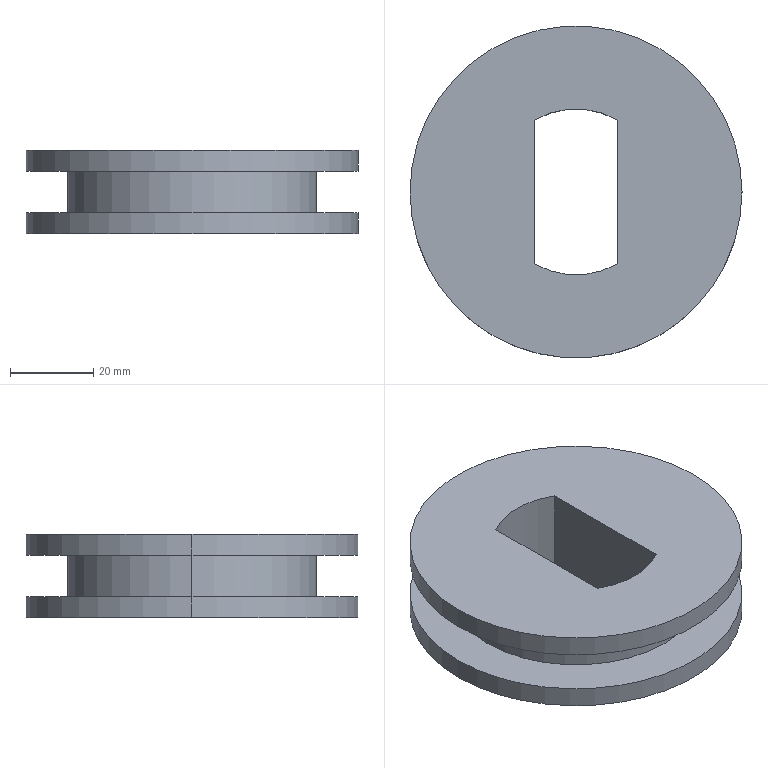Part | SolidWorks | 1 solid | 14 faces | box 80 x 80 x 20 mm | volume 63234 mm3 | cylinder 8 | plane 6 | commonest cylinder face diameters 80 x4 40 x2 60 x2
STEP:
#1=CARTESIAN_POINT('',(30.,0.,-5.));
#2=VERTEX_POINT('',#1);
#3=CARTESIAN_POINT('',(-30.,0.,-5.));
#4=VERTEX_POINT('',#3);
#5=CARTESIAN_POINT('',(0.,0.,-5.));
#6=DIRECTION('',(0.,0.,1.));
#7=DIRECTION('',(1.,0.,0.));
#8=AXIS2_PLACEMENT_3D('',#5,#6,#7);
#9=CIRCLE('',#8,30.);
#10=EDGE_CURVE('',#2,#4,#9,.T.);
#11=ORIENTED_EDGE('',*,*,#10,.T.);
#12=CARTESIAN_POINT('',(-30.,0.,5.));
#13=VERTEX_POINT('',#12);
#14=CARTESIAN_POINT('',(-30.,0.,10.));
#15=DIRECTION('',(0.,0.,1.));
#16=VECTOR('',#15,1000.);
#17=LINE('',#14,#16);
#18=EDGE_CURVE('',#4,#13,#17,.T.);
#19=ORIENTED_EDGE('',*,*,#18,.T.);
#20=CARTESIAN_POINT('',(30.,0.,5.));
#21=VERTEX_POINT('',#20);
#22=CARTESIAN_POINT('',(0.,0.,5.));
#23=DIRECTION('',(0.,0.,1.));
#24=DIRECTION('',(1.,0.,0.));
#25=AXIS2_PLACEMENT_3D('',#22,#23,#24);
#26=CIRCLE('',#25,30.);
#27=EDGE_CURVE('',#21,#13,#26,.T.);
#28=ORIENTED_EDGE('',*,*,#27,.F.);
#29=CARTESIAN_POINT('',(30.,0.,10.));
#30=DIRECTION('',(0.,0.,1.));
#31=VECTOR('',#30,1000.);
#32=LINE('',#29,#31);
#33=EDGE_CURVE('',#2,#21,#32,.T.);
#34=ORIENTED_EDGE('',*,*,#33,.F.);
#35=EDGE_LOOP('',(#11,#19,#28,#34));
#36=FACE_OUTER_BOUND('',#35,.T.);
#37=CARTESIAN_POINT('',(0.,0.,10.));
#38=DIRECTION('',(0.,0.,1.));
#39=DIRECTION('',(1.,0.,0.));
#40=AXIS2_PLACEMENT_3D('',#37,#38,#39);
#41=CYLINDRICAL_SURFACE('',#40,30.);
#42=ADVANCED_FACE('',(#36),#41,.T.);
#43=CARTESIAN_POINT('',(40.,0.,10.));
#44=VERTEX_POINT('',#43);
#45=CARTESIAN_POINT('',(-40.,0.,10.));
#46=VERTEX_POINT('',#45);
#47=CARTESIAN_POINT('',(0.,0.,10.));
#48=DIRECTION('',(0.,0.,1.));
#49=DIRECTION('',(1.,0.,0.));
#50=AXIS2_PLACEMENT_3D('',#47,#48,#49);
#51=CIRCLE('',#50,40.);
#52=EDGE_CURVE('',#44,#46,#51,.T.);
#53=ORIENTED_EDGE('',*,*,#52,.F.);
#54=CARTESIAN_POINT('',(40.,0.,5.));
#55=VERTEX_POINT('',#54);
#56=CARTESIAN_POINT('',(40.,0.,10.));
#57=DIRECTION('',(0.,0.,-1.));
#58=VECTOR('',#57,1000.);
#59=LINE('',#56,#58);
#60=EDGE_CURVE('',#44,#55,#59,.T.);
#61=ORIENTED_EDGE('',*,*,#60,.T.);
#62=CARTESIAN_POINT('',(-40.,0.,5.));
#63=VERTEX_POINT('',#62);
#64=CARTESIAN_POINT('',(0.,0.,5.));
#65=DIRECTION('',(0.,0.,-1.));
#66=DIRECTION('',(-1.,0.,0.));
#67=AXIS2_PLACEMENT_3D('',#64,#65,#66);
#68=CIRCLE('',#67,40.);
#69=EDGE_CURVE('',#63,#55,#68,.T.);
#70=ORIENTED_EDGE('',*,*,#69,.F.);
#71=CARTESIAN_POINT('',(-40.,0.,10.));
#72=DIRECTION('',(0.,0.,-1.));
#73=VECTOR('',#72,1000.);
#74=LINE('',#71,#73);
#75=EDGE_CURVE('',#46,#63,#74,.T.);
#76=ORIENTED_EDGE('',*,*,#75,.F.);
#77=EDGE_LOOP('',(#53,#61,#70,#76));
#78=FACE_OUTER_BOUND('',#77,.T.);
#79=CARTESIAN_POINT('',(0.,0.,10.));
#80=DIRECTION('',(0.,0.,-1.));
#81=DIRECTION('',(-1.,0.,0.));
#82=AXIS2_PLACEMENT_3D('',#79,#80,#81);
#83=CYLINDRICAL_SURFACE('',#82,40.);
#84=ADVANCED_FACE('',(#78),#83,.T.);
#85=CARTESIAN_POINT('',(40.,0.,-5.));
#86=VERTEX_POINT('',#85);
#87=CARTESIAN_POINT('',(-40.,0.,-5.));
#88=VERTEX_POINT('',#87);
#89=CARTESIAN_POINT('',(0.,0.,-5.));
#90=DIRECTION('',(0.,0.,1.));
#91=DIRECTION('',(1.,0.,0.));
#92=AXIS2_PLACEMENT_3D('',#89,#90,#91);
#93=CIRCLE('',#92,40.);
#94=EDGE_CURVE('',#86,#88,#93,.T.);
#95=ORIENTED_EDGE('',*,*,#94,.F.);
#96=CARTESIAN_POINT('',(40.,0.,-10.));
#97=VERTEX_POINT('',#96);
#98=CARTESIAN_POINT('',(40.,0.,10.));
#99=DIRECTION('',(0.,0.,-1.));
#100=VECTOR('',#99,1000.);
#101=LINE('',#98,#100);
#102=EDGE_CURVE('',#86,#97,#101,.T.);
#103=ORIENTED_EDGE('',*,*,#102,.T.);
#104=CARTESIAN_POINT('',(-40.,0.,-10.));
#105=VERTEX_POINT('',#104);
#106=CARTESIAN_POINT('',(0.,0.,-10.));
#107=DIRECTION('',(0.,0.,1.));
#108=DIRECTION('',(1.,0.,0.));
#109=AXIS2_PLACEMENT_3D('',#106,#107,#108);
#110=CIRCLE('',#109,40.);
#111=EDGE_CURVE('',#97,#105,#110,.T.);
#112=ORIENTED_EDGE('',*,*,#111,.T.);
#113=CARTESIAN_POINT('',(-40.,0.,10.));
#114=DIRECTION('',(0.,0.,-1.));
#115=VECTOR('',#114,1000.);
#116=LINE('',#113,#115);
#117=EDGE_CURVE('',#88,#105,#116,.T.);
#118=ORIENTED_EDGE('',*,*,#117,.F.);
#119=EDGE_LOOP('',(#95,#103,#112,#118));
#120=FACE_OUTER_BOUND('',#119,.T.);
#121=CARTESIAN_POINT('',(0.,0.,10.));
#122=DIRECTION('',(0.,0.,-1.));
#123=DIRECTION('',(-1.,0.,0.));
#124=AXIS2_PLACEMENT_3D('',#121,#122,#123);
#125=CYLINDRICAL_SURFACE('',#124,40.);
#126=ADVANCED_FACE('',(#120),#125,.T.);
#127=ORIENTED_EDGE('',*,*,#102,.F.);
#128=CARTESIAN_POINT('',(0.,0.,-5.));
#129=DIRECTION('',(0.,0.,1.));
#130=DIRECTION('',(1.,0.,0.));
#131=AXIS2_PLACEMENT_3D('',#128,#129,#130);
#132=CIRCLE('',#131,40.);
#133=EDGE_CURVE('',#88,#86,#132,.T.);
#134=ORIENTED_EDGE('',*,*,#133,.F.);
#135=ORIENTED_EDGE('',*,*,#117,.T.);
#136=CARTESIAN_POINT('',(0.,0.,-10.));
#137=DIRECTION('',(0.,0.,1.));
#138=DIRECTION('',(1.,0.,0.));
#139=AXIS2_PLACEMENT_3D('',#136,#137,#138);
#140=CIRCLE('',#139,40.);
#141=EDGE_CURVE('',#105,#97,#140,.T.);
#142=ORIENTED_EDGE('',*,*,#141,.T.);
#143=EDGE_LOOP('',(#127,#134,#135,#142));
#144=FACE_OUTER_BOUND('',#143,.T.);
#145=CARTESIAN_POINT('',(0.,0.,10.));
#146=DIRECTION('',(0.,0.,-1.));
#147=DIRECTION('',(-1.,0.,0.));
#148=AXIS2_PLACEMENT_3D('',#145,#146,#147);
#149=CYLINDRICAL_SURFACE('',#148,40.);
#150=ADVANCED_FACE('',(#144),#149,.T.);
#151=ORIENTED_EDGE('',*,*,#60,.F.);
#152=CARTESIAN_POINT('',(0.,0.,10.));
#153=DIRECTION('',(0.,0.,1.));
#154=DIRECTION('',(1.,0.,0.));
#155=AXIS2_PLACEMENT_3D('',#152,#153,#154);
#156=CIRCLE('',#155,40.);
#157=EDGE_CURVE('',#46,#44,#156,.T.);
#158=ORIENTED_EDGE('',*,*,#157,.F.);
#159=ORIENTED_EDGE('',*,*,#75,.T.);
#160=CARTESIAN_POINT('',(0.,0.,5.));
#161=DIRECTION('',(0.,0.,-1.));
#162=DIRECTION('',(-1.,0.,0.));
#163=AXIS2_PLACEMENT_3D('',#160,#161,#162);
#164=CIRCLE('',#163,40.);
#165=EDGE_CURVE('',#55,#63,#164,.T.);
#166=ORIENTED_EDGE('',*,*,#165,.F.);
#167=EDGE_LOOP('',(#151,#158,#159,#166));
#168=FACE_OUTER_BOUND('',#167,.T.);
#169=CARTESIAN_POINT('',(0.,0.,10.));
#170=DIRECTION('',(0.,0.,-1.));
#171=DIRECTION('',(-1.,0.,0.));
#172=AXIS2_PLACEMENT_3D('',#169,#170,#171);
#173=CYLINDRICAL_SURFACE('',#172,40.);
#174=ADVANCED_FACE('',(#168),#173,.T.);
#175=CARTESIAN_POINT('',(10.,17.321,-10.));
#176=VERTEX_POINT('',#175);
#177=CARTESIAN_POINT('',(-10.,17.321,-10.));
#178=VERTEX_POINT('',#177);
#179=CARTESIAN_POINT('',(0.,0.,-10.));
#180=DIRECTION('',(0.,0.,1.));
#181=DIRECTION('',(1.,0.,0.));
#182=AXIS2_PLACEMENT_3D('',#179,#180,#181);
#183=CIRCLE('',#182,20.);
#184=EDGE_CURVE('',#176,#178,#183,.T.);
#185=ORIENTED_EDGE('',*,*,#184,.F.);
#186=CARTESIAN_POINT('',(10.,17.321,10.));
#187=VERTEX_POINT('',#186);
#188=CARTESIAN_POINT('',(10.,17.321,10.));
#189=DIRECTION('',(0.,0.,-1.));
#190=VECTOR('',#189,1000.);
#191=LINE('',#188,#190);
#192=EDGE_CURVE('',#187,#176,#191,.T.);
#193=ORIENTED_EDGE('',*,*,#192,.F.);
#194=CARTESIAN_POINT('',(-10.,17.321,10.));
#195=VERTEX_POINT('',#194);
#196=CARTESIAN_POINT('',(0.,0.,10.));
#197=DIRECTION('',(0.,0.,1.));
#198=DIRECTION('',(1.,0.,0.));
#199=AXIS2_PLACEMENT_3D('',#196,#197,#198);
#200=CIRCLE('',#199,20.);
#201=EDGE_CURVE('',#187,#195,#200,.T.);
#202=ORIENTED_EDGE('',*,*,#201,.T.);
#203=CARTESIAN_POINT('',(-10.,17.321,10.));
#204=DIRECTION('',(0.,0.,-1.));
#205=VECTOR('',#204,1000.);
#206=LINE('',#203,#205);
#207=EDGE_CURVE('',#195,#178,#206,.T.);
#208=ORIENTED_EDGE('',*,*,#207,.T.);
#209=EDGE_LOOP('',(#185,#193,#202,#208));
#210=FACE_OUTER_BOUND('',#209,.T.);
#211=CARTESIAN_POINT('',(0.,0.,10.));
#212=DIRECTION('',(0.,0.,-1.));
#213=DIRECTION('',(-1.,0.,0.));
#214=AXIS2_PLACEMENT_3D('',#211,#212,#213);
#215=CYLINDRICAL_SURFACE('',#214,20.);
#216=ADVANCED_FACE('',(#210),#215,.F.);
#217=CARTESIAN_POINT('',(10.,-17.321,-10.));
#218=VERTEX_POINT('',#217);
#219=CARTESIAN_POINT('',(10.,0.,-10.));
#220=DIRECTION('',(0.,-1.,0.));
#221=VECTOR('',#220,1000.);
#222=LINE('',#219,#221);
#223=EDGE_CURVE('',#176,#218,#222,.T.);
#224=ORIENTED_EDGE('',*,*,#223,.T.);
#225=CARTESIAN_POINT('',(10.,-17.321,10.));
#226=VERTEX_POINT('',#225);
#227=CARTESIAN_POINT('',(10.,-17.321,10.));
#228=DIRECTION('',(0.,0.,-1.));
#229=VECTOR('',#228,1000.);
#230=LINE('',#227,#229);
#231=EDGE_CURVE('',#226,#218,#230,.T.);
#232=ORIENTED_EDGE('',*,*,#231,.F.);
#233=CARTESIAN_POINT('',(10.,0.,10.));
#234=DIRECTION('',(0.,-1.,0.));
#235=VECTOR('',#234,1000.);
#236=LINE('',#233,#235);
#237=EDGE_CURVE('',#187,#226,#236,.T.);
#238=ORIENTED_EDGE('',*,*,#237,.F.);
#239=ORIENTED_EDGE('',*,*,#192,.T.);
#240=EDGE_LOOP('',(#224,#232,#238,#239));
#241=FACE_OUTER_BOUND('',#240,.T.);
#242=CARTESIAN_POINT('',(10.,0.,10.));
#243=DIRECTION('',(1.,0.,0.));
#244=DIRECTION('',(0.,0.,-1.));
#245=AXIS2_PLACEMENT_3D('',#242,#243,#244);
#246=PLANE('',#245);
#247=ADVANCED_FACE('',(#241),#246,.F.);
#248=CARTESIAN_POINT('',(-10.,-17.321,-10.));
#249=VERTEX_POINT('',#248);
#250=CARTESIAN_POINT('',(0.,0.,-10.));
#251=DIRECTION('',(0.,0.,1.));
#252=DIRECTION('',(1.,0.,0.));
#253=AXIS2_PLACEMENT_3D('',#250,#251,#252);
#254=CIRCLE('',#253,20.);
#255=EDGE_CURVE('',#249,#218,#254,.T.);
#256=ORIENTED_EDGE('',*,*,#255,.F.);
#257=CARTESIAN_POINT('',(-10.,-17.321,10.));
#258=VERTEX_POINT('',#257);
#259=CARTESIAN_POINT('',(-10.,-17.321,10.));
#260=DIRECTION('',(0.,0.,-1.));
#261=VECTOR('',#260,1000.);
#262=LINE('',#259,#261);
#263=EDGE_CURVE('',#258,#249,#262,.T.);
#264=ORIENTED_EDGE('',*,*,#263,.F.);
#265=CARTESIAN_POINT('',(0.,0.,10.));
#266=DIRECTION('',(0.,0.,1.));
#267=DIRECTION('',(1.,0.,0.));
#268=AXIS2_PLACEMENT_3D('',#265,#266,#267);
#269=CIRCLE('',#268,20.);
#270=EDGE_CURVE('',#258,#226,#269,.T.);
#271=ORIENTED_EDGE('',*,*,#270,.T.);
#272=ORIENTED_EDGE('',*,*,#231,.T.);
#273=EDGE_LOOP('',(#256,#264,#271,#272));
#274=FACE_OUTER_BOUND('',#273,.T.);
#275=CARTESIAN_POINT('',(0.,0.,10.));
#276=DIRECTION('',(0.,0.,-1.));
#277=DIRECTION('',(-1.,0.,0.));
#278=AXIS2_PLACEMENT_3D('',#275,#276,#277);
#279=CYLINDRICAL_SURFACE('',#278,20.);
#280=ADVANCED_FACE('',(#274),#279,.F.);
#281=CARTESIAN_POINT('',(-10.,0.,-10.));
#282=DIRECTION('',(0.,-1.,0.));
#283=VECTOR('',#282,1000.);
#284=LINE('',#281,#283);
#285=EDGE_CURVE('',#178,#249,#284,.T.);
#286=ORIENTED_EDGE('',*,*,#285,.F.);
#287=ORIENTED_EDGE('',*,*,#207,.F.);
#288=CARTESIAN_POINT('',(-10.,0.,10.));
#289=DIRECTION('',(0.,-1.,0.));
#290=VECTOR('',#289,1000.);
#291=LINE('',#288,#290);
#292=EDGE_CURVE('',#195,#258,#291,.T.);
#293=ORIENTED_EDGE('',*,*,#292,.T.);
#294=ORIENTED_EDGE('',*,*,#263,.T.);
#295=EDGE_LOOP('',(#286,#287,#293,#294));
#296=FACE_OUTER_BOUND('',#295,.T.);
#297=CARTESIAN_POINT('',(-10.,0.,10.));
#298=DIRECTION('',(1.,0.,0.));
#299=DIRECTION('',(0.,0.,-1.));
#300=AXIS2_PLACEMENT_3D('',#297,#298,#299);
#301=PLANE('',#300);
#302=ADVANCED_FACE('',(#296),#301,.T.);
#303=ORIENTED_EDGE('',*,*,#201,.F.);
#304=ORIENTED_EDGE('',*,*,#237,.T.);
#305=ORIENTED_EDGE('',*,*,#270,.F.);
#306=ORIENTED_EDGE('',*,*,#292,.F.);
#307=EDGE_LOOP('',(#303,#304,#305,#306));
#308=FACE_BOUND('',#307,.T.);
#309=ORIENTED_EDGE('',*,*,#157,.T.);
#310=ORIENTED_EDGE('',*,*,#52,.T.);
#311=EDGE_LOOP('',(#309,#310));
#312=FACE_OUTER_BOUND('',#311,.T.);
#313=CARTESIAN_POINT('',(0.,0.,10.));
#314=DIRECTION('',(0.,0.,1.));
#315=DIRECTION('',(1.,0.,0.));
#316=AXIS2_PLACEMENT_3D('',#313,#314,#315);
#317=PLANE('',#316);
#318=ADVANCED_FACE('',(#308,#312),#317,.T.);
#319=ORIENTED_EDGE('',*,*,#184,.T.);
#320=ORIENTED_EDGE('',*,*,#285,.T.);
#321=ORIENTED_EDGE('',*,*,#255,.T.);
#322=ORIENTED_EDGE('',*,*,#223,.F.);
#323=EDGE_LOOP('',(#319,#320,#321,#322));
#324=FACE_BOUND('',#323,.T.);
#325=ORIENTED_EDGE('',*,*,#141,.F.);
#326=ORIENTED_EDGE('',*,*,#111,.F.);
#327=EDGE_LOOP('',(#325,#326));
#328=FACE_OUTER_BOUND('',#327,.T.);
#329=CARTESIAN_POINT('',(0.,0.,-10.));
#330=DIRECTION('',(0.,0.,1.));
#331=DIRECTION('',(1.,0.,0.));
#332=AXIS2_PLACEMENT_3D('',#329,#330,#331);
#333=PLANE('',#332);
#334=ADVANCED_FACE('',(#324,#328),#333,.F.);
#335=ORIENTED_EDGE('',*,*,#10,.F.);
#336=CARTESIAN_POINT('',(0.,0.,-5.));
#337=DIRECTION('',(0.,0.,1.));
#338=DIRECTION('',(1.,0.,0.));
#339=AXIS2_PLACEMENT_3D('',#336,#337,#338);
#340=CIRCLE('',#339,30.);
#341=EDGE_CURVE('',#4,#2,#340,.T.);
#342=ORIENTED_EDGE('',*,*,#341,.F.);
#343=EDGE_LOOP('',(#335,#342));
#344=FACE_BOUND('',#343,.T.);
#345=ORIENTED_EDGE('',*,*,#133,.T.);
#346=ORIENTED_EDGE('',*,*,#94,.T.);
#347=EDGE_LOOP('',(#345,#346));
#348=FACE_OUTER_BOUND('',#347,.T.);
#349=CARTESIAN_POINT('',(0.,50.,-5.));
#350=DIRECTION('',(0.,0.,1.));
#351=DIRECTION('',(1.,0.,0.));
#352=AXIS2_PLACEMENT_3D('',#349,#350,#351);
#353=PLANE('',#352);
#354=ADVANCED_FACE('',(#344,#348),#353,.T.);
#355=ORIENTED_EDGE('',*,*,#27,.T.);
#356=CARTESIAN_POINT('',(0.,0.,5.));
#357=DIRECTION('',(0.,0.,1.));
#358=DIRECTION('',(1.,0.,0.));
#359=AXIS2_PLACEMENT_3D('',#356,#357,#358);
#360=CIRCLE('',#359,30.);
#361=EDGE_CURVE('',#13,#21,#360,.T.);
#362=ORIENTED_EDGE('',*,*,#361,.T.);
#363=EDGE_LOOP('',(#355,#362));
#364=FACE_BOUND('',#363,.T.);
#365=ORIENTED_EDGE('',*,*,#69,.T.);
#366=ORIENTED_EDGE('',*,*,#165,.T.);
#367=EDGE_LOOP('',(#365,#366));
#368=FACE_OUTER_BOUND('',#367,.T.);
#369=CARTESIAN_POINT('',(0.,50.,5.));
#370=DIRECTION('',(0.,0.,-1.));
#371=DIRECTION('',(-1.,0.,0.));
#372=AXIS2_PLACEMENT_3D('',#369,#370,#371);
#373=PLANE('',#372);
#374=ADVANCED_FACE('',(#364,#368),#373,.T.);
#375=ORIENTED_EDGE('',*,*,#18,.F.);
#376=ORIENTED_EDGE('',*,*,#341,.T.);
#377=ORIENTED_EDGE('',*,*,#33,.T.);
#378=ORIENTED_EDGE('',*,*,#361,.F.);
#379=EDGE_LOOP('',(#375,#376,#377,#378));
#380=FACE_OUTER_BOUND('',#379,.T.);
#381=CARTESIAN_POINT('',(0.,0.,10.));
#382=DIRECTION('',(0.,0.,1.));
#383=DIRECTION('',(1.,0.,0.));
#384=AXIS2_PLACEMENT_3D('',#381,#382,#383);
#385=CYLINDRICAL_SURFACE('',#384,30.);
#386=ADVANCED_FACE('',(#380),#385,.T.);
#387=CLOSED_SHELL('',(#42,#84,#126,#150,#174,#216,#247,#280,#302,#318,#334,#354,#374,#386));
#388=MANIFOLD_SOLID_BREP('',#387);
#389=CARTESIAN_POINT('',(0.,0.,0.));
#390=DIRECTION('',(0.,0.,1.));
#391=DIRECTION('',(1.,0.,0.));
#392=AXIS2_PLACEMENT_3D('',#389,#390,#391);
#393=(LENGTH_UNIT()NAMED_UNIT(*)SI_UNIT(.MILLI.,.METRE.));
#394=UNCERTAINTY_MEASURE_WITH_UNIT(LENGTH_MEASURE(0.00001),#393,'','');
#395=(NAMED_UNIT(*)PLANE_ANGLE_UNIT()SI_UNIT($,.RADIAN.));
#396=(NAMED_UNIT(*)SI_UNIT($,.STERADIAN.)SOLID_ANGLE_UNIT());
#397=(GEOMETRIC_REPRESENTATION_CONTEXT(3)GLOBAL_UNCERTAINTY_ASSIGNED_CONTEXT((#394))GLOBAL_UNIT_ASSIGNED_CONTEXT((#393,#395,#396))REPRESENTATION_CONTEXT('',''));
#398=ADVANCED_BREP_SHAPE_REPRESENTATION('',(#388,#392),#397);